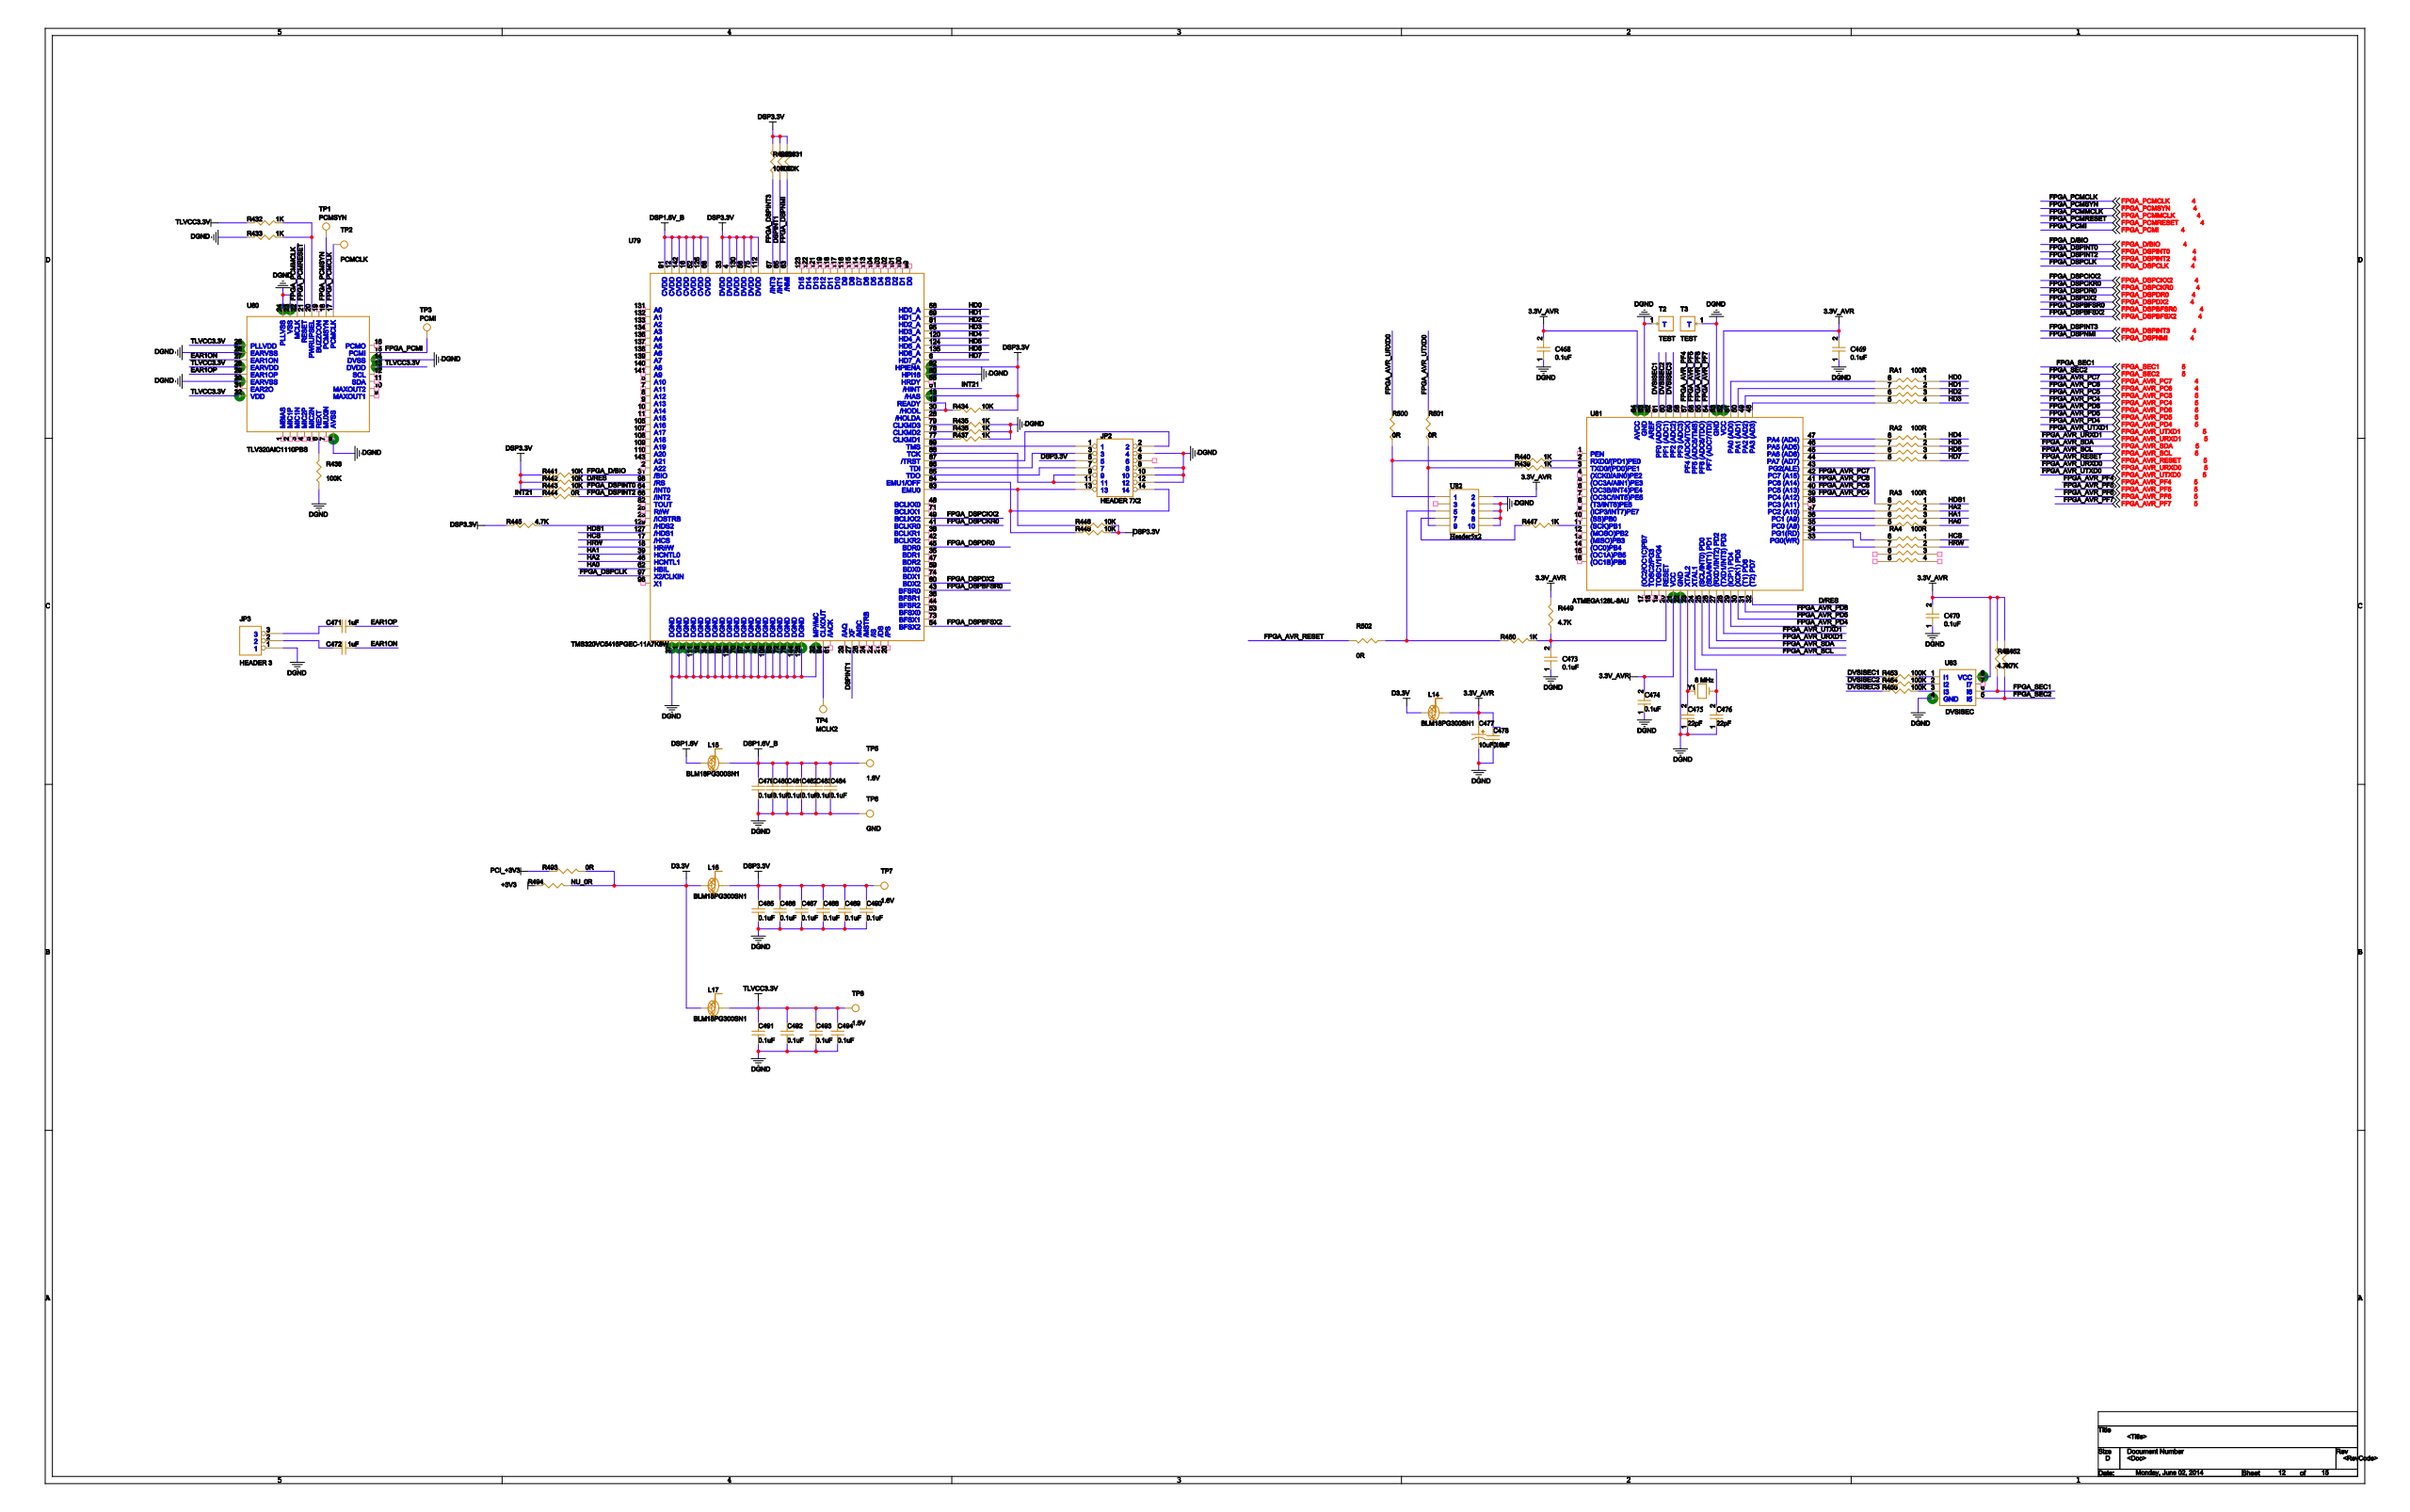Circuit board | Cadence Allegro | 669 parts | 806 nets | one sheet of the schematic
Parts on this sheet (reference | value | footprint):
C468 | 0.1uF | C0402
C469 | 0.1uF | C0402
C470 | 0.1uF | C0402
C471 | 1uF | C0603
C472 | 1uF | C0603
C473 | 0.1uF | C0402
C474 | 0.1uF | C0402
C475 | 22pF | C0402
C476 | 22pF | C0402
C477 | 10uF,16V | CP3216
C478 | 0.1uF | C0402
C479 | 0.1uF | C0402
C480 | 0.1uF | C0402
C481 | 0.1uF | C0402
C482 | 0.1uF | C0402
C483 | 0.1uF | C0402
C484 | 0.1uF | C0402
C485 | 0.1uF | C0402
C486 | 0.1uF | C0402
C487 | 0.1uF | C0402
C488 | 0.1uF | C0402
C489 | 0.1uF | C0402
C490 | 0.1uF | C0402
C491 | 0.1uF | C0402
C492 | 0.1uF | C0402
C493 | 0.1uF | C0402
C494 | 0.1uF | C0402
JP2 | HEADER 7X2 | ZIP14
JP3 | HEADER 3 | SIP3
L14 | BLM18PG300SN1 | F0603
L15 | BLM18PG300SN1 | F0603
L16 | BLM18PG300SN1 | F0603
L17 | BLM18PG300SN1 | F0603
R429 | 10K | R0603
R430 | 10K | R0603
R431 | 10K | R0603
R432 | 1K | R0603
R433 | 1K | R0603
R434 | 10K | R0603
R435 | 1K | R0603
R436 | 1K | R0603
R437 | 1K | R0603
R438 | 100K | R0603
R439 | 1K | R0603
R440 | 1K | R0603
R441 | 10K | R0603
R442 | 10K | R0603
R443 | 10K | R0603
R444 | 0R | R0603
R445 | 4.7K | R0603
R446 | 10K | R0603
R447 | 1K | R0603
R448 | 10K | R0603
R449 | 4.7K | R0603
R450 | 1K | R0603
R451 | 4.7K | R0603
R452 | 4.7K | R0603
R453 | 100K | R0603
R454 | 100K | R0603
R455 | 100K | R0603
R493 | 0R | R1210
R494 | NU_0R | R1210
R500 | 0R | R0603
R501 | 0R | R0603
R502 | 0R | R0603
RA1 | 100R | 8P4R0603
RA2 | 100R | 8P4R0603
RA3 | 100R | 8P4R0603
RA4 | 100R | 8P4R0603
T3 | TEST | SMD1
TP1 | PCMSYN | SIP1
TP2 | PCMCLK | SIP1
TP3 | PCMI | SIP1
TP4 | MCLK2 | SIP1
TP5 | 1.6V | SIP1
TP6 | GND | SIP1
TP7 | 1.6V | SIP1
TP8 | 1.6V | SIP1
U79 | TMS320VC5416PGEC-11A7K8W | QFP144_0P5M_22X22M
U80 | TLV320AIC1110PBS | QFP32_0P5M_7X7M
U81 | ATMEGA128L-8AU | QFP64_0P8M_16X16M
U82 | Header5x2 | ZIP10
U83 | DVSISEC | SOP8_1P27M_6X5M
Nets of these parts (net: part-pin ...):
DGND: C468-1 C469-1 C470-1 C473-1 C474-1 C475-1 C476-1 C477-2 C478-2 C479-2 C480-2 C481-2 C482-2 C483-2 C484-2 C485-2 C486-2 C487-2 C488-2 C489-2 C490-2 C491-2 C492-2 C493-2 C494-2 JP2-4 JP2-8 JP2-10 JP2-12 JP3-1 R433-1 R435-2 R436-2 R437-2 R438-1 T3-1 TP6-1 U80-8 U80-14 U80-23 U80-24 U80-26 U80-30 U82-4 U82-6 U82-8 U82-10 U83-4 U79-1 U79-3 U79-14 U79-15 U79-32 U79-34 U79-37 U79-40 U79-50 U79-57 U79-70 U79-72 U79-76 U79-80 U79-90 U79-93 U79-106 U79-111 U79-126 U79-128 U79-144 U81-22 U81-53 U81-63
N60950508: R453-2 U83-1
N60950510: R454-2 U83-2
N60950512: R455-2 U83-3
FPGA_SEC2: R452-1 U83-5
FPGA_SEC1: R451-1 U83-6
3.3V_AVR: C468-2 C469-2 C470-2 C474-2 C477-1 C478-1 L14-2 R449-2 R451-2 R452-2 U82-2 U83-8 U81-21 U81-52 U81-64
+3V3: R494-1
FPGA_AVR_URXD1: U81-27
FPGA_PCMCLK: TP2-1 U80-17
FPGA_DSPCLK: U79-97
FPGA_AVR_PF6: U81-55
FPGA_PCMSYN: TP1-1 U80-18
FPGA_AVR_PC6: U81-41
FPGA_AVR_PC7: U81-42
FPGA_DSPCKX2: U79-49
FPGA_PCMMCLK: U80-22
FPGA_PCMRESET: U80-21
FPGA_AVR_URXD0: R500-2
FPGA_DSPBFSX2: U79-54
FPGA_PCMI: TP3-1 U80-15
FPGA_DSPINT3: R429-1 U79-67
FPGA_DSPDX2: U79-60
FPGA_DSPDR0: U79-45
FPGA_DSPCKR0: U79-41
FPGA_DSPBFSR0: U79-43
FPGA_DSPINT0: R443-2 U79-64
FPGA_D/BIO: R441-2 U79-31
FPGA_AVR_RESET: R502-2
FPGA_AVR_PF4: U81-57
FPGA_AVR_PF7: U81-54
FPGA_AVR_PC5: U81-40
FPGA_AVR_PF5: U81-56
FPGA_AVR_SCL: U81-25
FPGA_AVR_PC4: U81-39
FPGA_AVR_SDA: U81-26
FPGA_AVR_PD5: U81-30
FPGA_AVR_UTXD0: R501-2
FPGA_DSPNMI: R431-1 U79-63
FPGA_AVR_PD4: U81-29
FPGA_AVR_UTXD1: U81-28
FPGA_AVR_PD6: U81-31
FPGA_DSPINT2: R444-2 U79-66
TLVCC3.3V: C491-1 C492-1 C493-1 C494-1 L17-2 R432-1 TP8-1 U80-13 U80-25 U80-28 U80-32
EAR1ON: C472-2 U80-27
EAR1OP: C471-2 U80-29
N16273595: R432-2 R433-2 U80-20
N16272401: R438-2 U80-6
N60950764: R447-2 U81-11
D/RES: R442-2 U79-98 U81-32
N60950635: RA1-8 U81-51
N60950631: RA1-7 U81-50
N60950627: RA1-6 U81-49
N60950623: RA1-5 U81-48
N60950639: RA2-8 U81-47
N60950641: RA2-7 U81-46
N60950643: RA2-6 U81-45
N60950645: RA2-5 U81-44
N60950651: RA3-5 U81-35
N60950661: RA3-6 U81-36
N60950663: RA3-7 U81-37
DVSISEC1: R453-1 U81-61
DVSISEC2: R454-1 U81-60
DVSISEC3: R455-1 U81-59
N60950649: RA4-7 U81-33
N60950647: RA4-8 U81-34
N60950665: RA3-8 U81-43
N60950799: C473-2 R449-1 R450-2 U81-20
N60950742: R440-2 U81-2
N60950744: R439-2 U81-3
N60950506: C476-2 U81-24
N60950504: C475-2 U81-23
PCI_+3V3: R493-1
N60950750: R440-1 R500-1 U82-1
N60950757: R439-1 R501-1 U82-9
N60950792: R450-1 R502-1 U82-5
INT21: R444-1 U79-51
D3.3V: L14-1 L16-1 L17-1 R493-2 R494-2
HD0: RA1-1 U79-58
HD1: RA1-2 U79-69
HD2: RA1-3 U79-81
HD3: RA1-4 U79-95
HD4: RA2-1 U79-120
HD5: RA2-2 U79-124
HD6: RA2-3 U79-135
HD7: RA2-4 U79-6
HDS1: RA3-1 U79-127
HA2: RA3-2 U79-46
HA1: RA3-3 U79-39
HA0: RA3-4 U79-62
HCS: RA4-1 U79-17
HRW: RA4-2 U79-18
DSP3.3V: C485-1 C486-1 C487-1 C488-1 C489-1 C490-1 JP2-5 L16-2 R429-2 R430-2 R431-2 R434-2 R441-1 R442-1 R443-1 R445-1 R446-2 R448-2 TP7-1 U79-4 U79-13 U79-33 U79-56 U79-75 U79-92 U79-112 U79-130
N16287064: R445-2 U79-129
N16275556: R434-1 U79-19 U79-30
DSPINT1: R430-1 U79-27 U79-65
N16276075: JP2-2 U79-87
N16275770: R437-1 U79-77
N16275766: R436-1 U79-78
N16275762: R435-1 U79-79
N16279666: TP4-1 U79-94
DSP1.6V_B: C479-1 C480-1 C481-1 C482-1 C483-1 C484-1 L15-2 TP5-1 U79-12 U79-16 U79-52 U79-68 U79-91 U79-125 U79-142
N16276947: JP2-13 R446-1 U79-83
N16276922: JP2-14 R448-1 U79-84
N16276051: JP2-9 JP2-11 U79-88
N16276133: JP2-3 U79-86
N16276241: JP2-7 U79-85
N61571144: JP2-1 U79-89
N16278993: C471-1 JP3-3
N16278981: C472-1 JP3-2
N60950766: R447-1 U82-7
DSP1.6V: L15-1